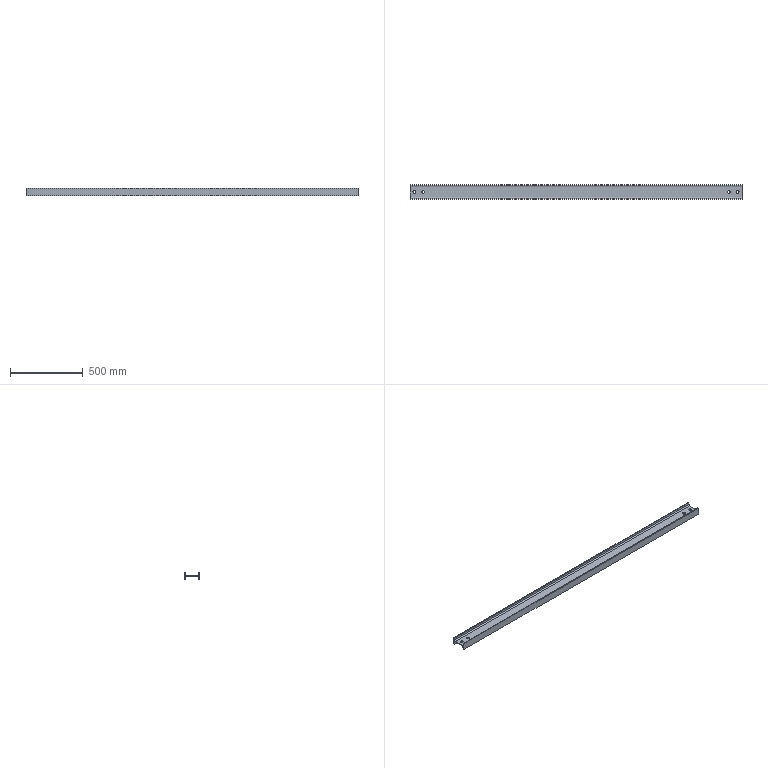Part | STEP file | 电柜辅梁1主体_Default<As Machined> | 1 solid | 26 faces | box 2280 x 100 x 50 mm | volume 2695988 mm3 | plane 14 | cylinder 12 | commonest cylinder face diameters 19 x8 16 x4